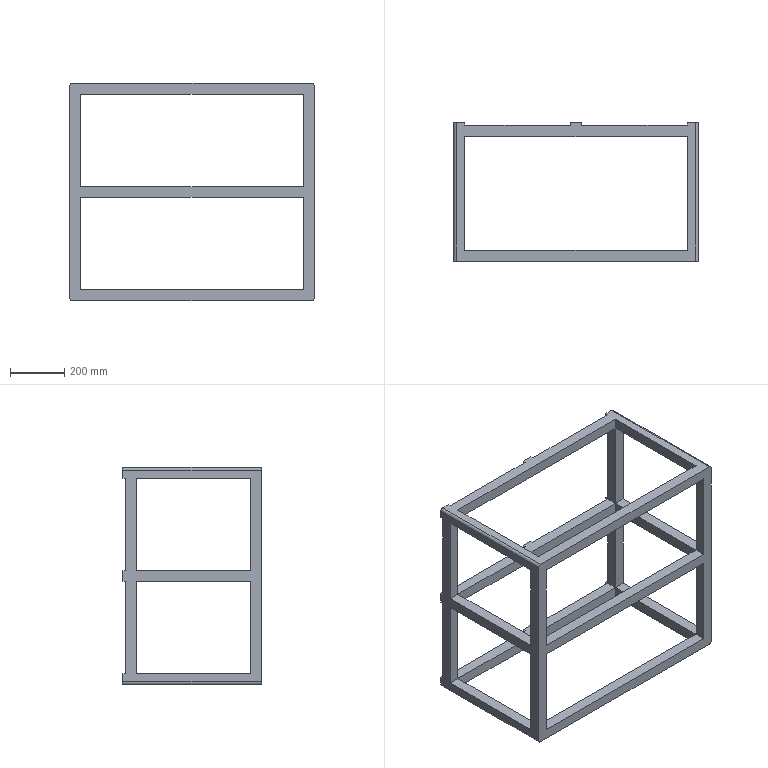Part | SolidWorks | features BaseBody 1 | 1 solid | 128 faces | box 900 x 510 x 800 mm | volume 17121482 mm3 | plane 88 | cylinder 22 | cone 18 | commonest cylinder face diameters 5 x18 20 x4